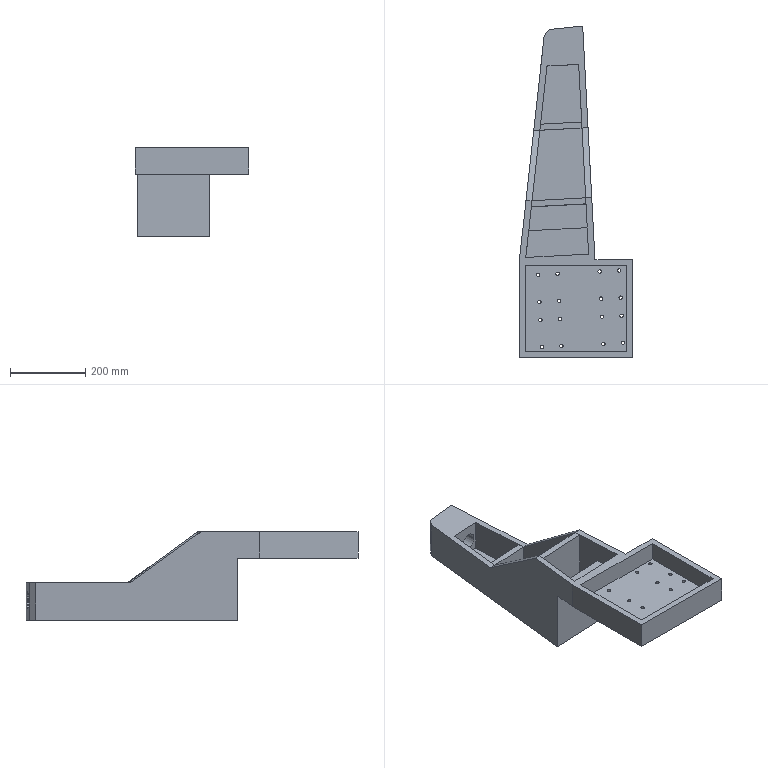Part | SolidWorks | features ICE 9, Chamfer 1, Cut 1, Extrusion 1, Shell 1, WeldmentFeature 1 | 3 solids | 73 faces | box 300 x 880.131 x 235 mm | volume 7902209 mm3 | plane 39 | cylinder 34 | commonest cylinder face diameters 9 x32 45 x2